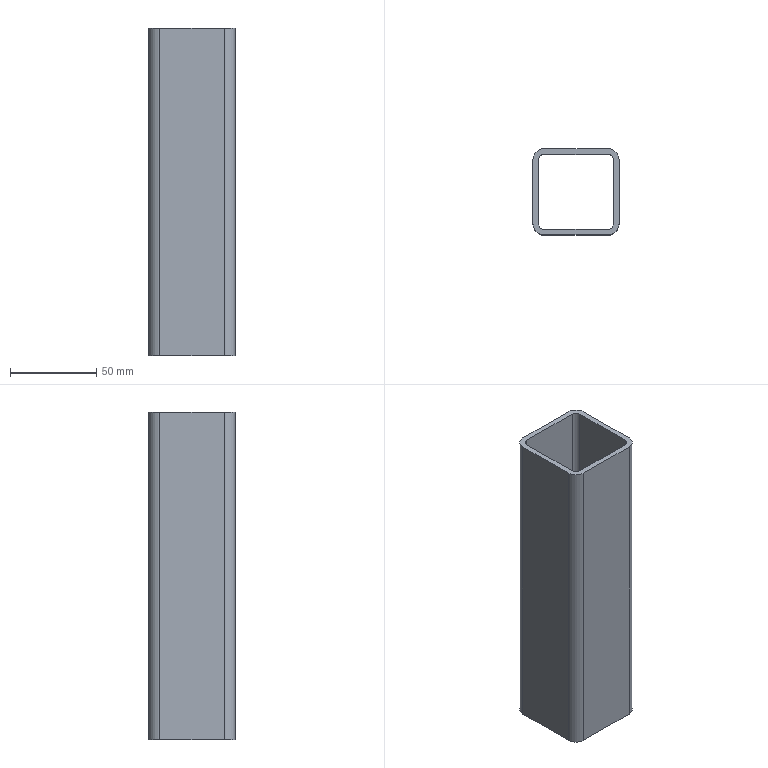Part | STEP file | JIS G 3466 50 x 50 x 3,2 1784904759157 | 1 solid | 18 faces | box 50 x 50 x 190 mm | volume 108807 mm3 | plane 10 | cylinder 8 | commonest cylinder face diameters 6.4 x4 12.8 x4
STEP:
#1=CARTESIAN_POINT('',(-18.6,-21.8,240.));
#2=VERTEX_POINT('',#1);
#3=CARTESIAN_POINT('',(18.6,-21.8,240.));
#4=VERTEX_POINT('',#3);
#5=CARTESIAN_POINT('',(9.3,-21.8,240.));
#6=DIRECTION('',(1.,0.,0.));
#7=VECTOR('',#6,10.);
#8=LINE('',#5,#7);
#9=EDGE_CURVE('',#2,#4,#8,.T.);
#10=ORIENTED_EDGE('',*,*,#9,.T.);
#11=CARTESIAN_POINT('',(18.6,-21.8,50.));
#12=VERTEX_POINT('',#11);
#13=CARTESIAN_POINT('',(18.6,-21.8,0.));
#14=DIRECTION('',(0.,0.,1.));
#15=VECTOR('',#14,10.);
#16=LINE('',#13,#15);
#17=EDGE_CURVE('',#12,#4,#16,.T.);
#18=ORIENTED_EDGE('',*,*,#17,.F.);
#19=CARTESIAN_POINT('',(-18.6,-21.8,50.));
#20=VERTEX_POINT('',#19);
#21=CARTESIAN_POINT('',(9.3,-21.8,50.));
#22=DIRECTION('',(1.,0.,0.));
#23=VECTOR('',#22,10.);
#24=LINE('',#21,#23);
#25=EDGE_CURVE('',#20,#12,#24,.T.);
#26=ORIENTED_EDGE('',*,*,#25,.F.);
#27=CARTESIAN_POINT('',(-18.6,-21.8,0.));
#28=DIRECTION('',(0.,0.,1.));
#29=VECTOR('',#28,10.);
#30=LINE('',#27,#29);
#31=EDGE_CURVE('',#20,#2,#30,.T.);
#32=ORIENTED_EDGE('',*,*,#31,.T.);
#33=EDGE_LOOP('',(#10,#18,#26,#32));
#34=FACE_OUTER_BOUND('',#33,.T.);
#35=CARTESIAN_POINT('',(18.6,-21.8,0.));
#36=DIRECTION('',(0.,-1.,0.));
#37=DIRECTION('',(0.,0.,-1.));
#38=AXIS2_PLACEMENT_3D('',#35,#36,#37);
#39=PLANE('',#38);
#40=ADVANCED_FACE('',(#34),#39,.F.);
#41=CARTESIAN_POINT('',(21.8,-18.6,240.));
#42=VERTEX_POINT('',#41);
#43=CARTESIAN_POINT('',(18.6,-18.6,240.));
#44=DIRECTION('',(0.,0.,1.));
#45=DIRECTION('',(0.,1.,0.));
#46=AXIS2_PLACEMENT_3D('',#43,#44,#45);
#47=CIRCLE('',#46,3.2);
#48=EDGE_CURVE('',#4,#42,#47,.T.);
#49=ORIENTED_EDGE('',*,*,#48,.T.);
#50=CARTESIAN_POINT('',(21.8,-18.6,50.));
#51=VERTEX_POINT('',#50);
#52=CARTESIAN_POINT('',(21.8,-18.6,0.));
#53=DIRECTION('',(0.,0.,1.));
#54=VECTOR('',#53,10.);
#55=LINE('',#52,#54);
#56=EDGE_CURVE('',#51,#42,#55,.T.);
#57=ORIENTED_EDGE('',*,*,#56,.F.);
#58=CARTESIAN_POINT('',(18.6,-18.6,50.));
#59=DIRECTION('',(0.,0.,1.));
#60=DIRECTION('',(0.,1.,0.));
#61=AXIS2_PLACEMENT_3D('',#58,#59,#60);
#62=CIRCLE('',#61,3.2);
#63=EDGE_CURVE('',#12,#51,#62,.T.);
#64=ORIENTED_EDGE('',*,*,#63,.F.);
#65=ORIENTED_EDGE('',*,*,#17,.T.);
#66=EDGE_LOOP('',(#49,#57,#64,#65));
#67=FACE_OUTER_BOUND('',#66,.T.);
#68=CARTESIAN_POINT('',(18.6,-18.6,0.));
#69=DIRECTION('',(0.,0.,1.));
#70=DIRECTION('',(0.,1.,0.));
#71=AXIS2_PLACEMENT_3D('',#68,#69,#70);
#72=CYLINDRICAL_SURFACE('',#71,3.2);
#73=ADVANCED_FACE('',(#67),#72,.F.);
#74=CARTESIAN_POINT('',(21.8,18.6,240.));
#75=VERTEX_POINT('',#74);
#76=CARTESIAN_POINT('',(21.8,9.3,240.));
#77=DIRECTION('',(0.,1.,0.));
#78=VECTOR('',#77,10.);
#79=LINE('',#76,#78);
#80=EDGE_CURVE('',#42,#75,#79,.T.);
#81=ORIENTED_EDGE('',*,*,#80,.T.);
#82=CARTESIAN_POINT('',(21.8,18.6,50.));
#83=VERTEX_POINT('',#82);
#84=CARTESIAN_POINT('',(21.8,18.6,0.));
#85=DIRECTION('',(0.,0.,1.));
#86=VECTOR('',#85,10.);
#87=LINE('',#84,#86);
#88=EDGE_CURVE('',#83,#75,#87,.T.);
#89=ORIENTED_EDGE('',*,*,#88,.F.);
#90=CARTESIAN_POINT('',(21.8,9.3,50.));
#91=DIRECTION('',(0.,1.,0.));
#92=VECTOR('',#91,10.);
#93=LINE('',#90,#92);
#94=EDGE_CURVE('',#51,#83,#93,.T.);
#95=ORIENTED_EDGE('',*,*,#94,.F.);
#96=ORIENTED_EDGE('',*,*,#56,.T.);
#97=EDGE_LOOP('',(#81,#89,#95,#96));
#98=FACE_OUTER_BOUND('',#97,.T.);
#99=CARTESIAN_POINT('',(21.8,18.6,0.));
#100=DIRECTION('',(1.,0.,0.));
#101=DIRECTION('',(0.,0.,-1.));
#102=AXIS2_PLACEMENT_3D('',#99,#100,#101);
#103=PLANE('',#102);
#104=ADVANCED_FACE('',(#98),#103,.F.);
#105=CARTESIAN_POINT('',(18.6,21.8,240.));
#106=VERTEX_POINT('',#105);
#107=CARTESIAN_POINT('',(18.6,18.6,240.));
#108=DIRECTION('',(0.,0.,1.));
#109=DIRECTION('',(-1.,0.,0.));
#110=AXIS2_PLACEMENT_3D('',#107,#108,#109);
#111=CIRCLE('',#110,3.2);
#112=EDGE_CURVE('',#75,#106,#111,.T.);
#113=ORIENTED_EDGE('',*,*,#112,.T.);
#114=CARTESIAN_POINT('',(18.6,21.8,50.));
#115=VERTEX_POINT('',#114);
#116=CARTESIAN_POINT('',(18.6,21.8,0.));
#117=DIRECTION('',(0.,0.,1.));
#118=VECTOR('',#117,10.);
#119=LINE('',#116,#118);
#120=EDGE_CURVE('',#115,#106,#119,.T.);
#121=ORIENTED_EDGE('',*,*,#120,.F.);
#122=CARTESIAN_POINT('',(18.6,18.6,50.));
#123=DIRECTION('',(0.,0.,1.));
#124=DIRECTION('',(-1.,0.,0.));
#125=AXIS2_PLACEMENT_3D('',#122,#123,#124);
#126=CIRCLE('',#125,3.2);
#127=EDGE_CURVE('',#83,#115,#126,.T.);
#128=ORIENTED_EDGE('',*,*,#127,.F.);
#129=ORIENTED_EDGE('',*,*,#88,.T.);
#130=EDGE_LOOP('',(#113,#121,#128,#129));
#131=FACE_OUTER_BOUND('',#130,.T.);
#132=CARTESIAN_POINT('',(18.6,18.6,0.));
#133=DIRECTION('',(0.,0.,1.));
#134=DIRECTION('',(-1.,0.,0.));
#135=AXIS2_PLACEMENT_3D('',#132,#133,#134);
#136=CYLINDRICAL_SURFACE('',#135,3.2);
#137=ADVANCED_FACE('',(#131),#136,.F.);
#138=CARTESIAN_POINT('',(25.,18.6,240.));
#139=VERTEX_POINT('',#138);
#140=CARTESIAN_POINT('',(25.,-18.6,240.));
#141=VERTEX_POINT('',#140);
#142=CARTESIAN_POINT('',(25.,9.3,240.));
#143=DIRECTION('',(0.,-1.,0.));
#144=VECTOR('',#143,10.);
#145=LINE('',#142,#144);
#146=EDGE_CURVE('',#139,#141,#145,.T.);
#147=ORIENTED_EDGE('',*,*,#146,.T.);
#148=CARTESIAN_POINT('',(25.,-18.6,50.));
#149=VERTEX_POINT('',#148);
#150=CARTESIAN_POINT('',(25.,-18.6,0.));
#151=DIRECTION('',(0.,0.,1.));
#152=VECTOR('',#151,10.);
#153=LINE('',#150,#152);
#154=EDGE_CURVE('',#149,#141,#153,.T.);
#155=ORIENTED_EDGE('',*,*,#154,.F.);
#156=CARTESIAN_POINT('',(25.,18.6,50.));
#157=VERTEX_POINT('',#156);
#158=CARTESIAN_POINT('',(25.,9.3,50.));
#159=DIRECTION('',(0.,-1.,0.));
#160=VECTOR('',#159,10.);
#161=LINE('',#158,#160);
#162=EDGE_CURVE('',#157,#149,#161,.T.);
#163=ORIENTED_EDGE('',*,*,#162,.F.);
#164=CARTESIAN_POINT('',(25.,18.6,0.));
#165=DIRECTION('',(0.,0.,1.));
#166=VECTOR('',#165,10.);
#167=LINE('',#164,#166);
#168=EDGE_CURVE('',#157,#139,#167,.T.);
#169=ORIENTED_EDGE('',*,*,#168,.T.);
#170=EDGE_LOOP('',(#147,#155,#163,#169));
#171=FACE_OUTER_BOUND('',#170,.T.);
#172=CARTESIAN_POINT('',(25.,18.6,0.));
#173=DIRECTION('',(1.,0.,0.));
#174=DIRECTION('',(0.,0.,-1.));
#175=AXIS2_PLACEMENT_3D('',#172,#173,#174);
#176=PLANE('',#175);
#177=ADVANCED_FACE('',(#171),#176,.T.);
#178=CARTESIAN_POINT('',(18.6,-25.,240.));
#179=VERTEX_POINT('',#178);
#180=CARTESIAN_POINT('',(18.6,-18.6,240.));
#181=DIRECTION('',(0.,0.,-1.));
#182=DIRECTION('',(0.,1.,0.));
#183=AXIS2_PLACEMENT_3D('',#180,#181,#182);
#184=CIRCLE('',#183,6.4);
#185=EDGE_CURVE('',#141,#179,#184,.T.);
#186=ORIENTED_EDGE('',*,*,#185,.T.);
#187=CARTESIAN_POINT('',(18.6,-25.,50.));
#188=VERTEX_POINT('',#187);
#189=CARTESIAN_POINT('',(18.6,-25.,0.));
#190=DIRECTION('',(0.,0.,1.));
#191=VECTOR('',#190,10.);
#192=LINE('',#189,#191);
#193=EDGE_CURVE('',#188,#179,#192,.T.);
#194=ORIENTED_EDGE('',*,*,#193,.F.);
#195=CARTESIAN_POINT('',(18.6,-18.6,50.));
#196=DIRECTION('',(0.,0.,-1.));
#197=DIRECTION('',(0.,1.,0.));
#198=AXIS2_PLACEMENT_3D('',#195,#196,#197);
#199=CIRCLE('',#198,6.4);
#200=EDGE_CURVE('',#149,#188,#199,.T.);
#201=ORIENTED_EDGE('',*,*,#200,.F.);
#202=ORIENTED_EDGE('',*,*,#154,.T.);
#203=EDGE_LOOP('',(#186,#194,#201,#202));
#204=FACE_OUTER_BOUND('',#203,.T.);
#205=CARTESIAN_POINT('',(18.6,-18.6,0.));
#206=DIRECTION('',(0.,0.,1.));
#207=DIRECTION('',(0.,1.,0.));
#208=AXIS2_PLACEMENT_3D('',#205,#206,#207);
#209=CYLINDRICAL_SURFACE('',#208,6.4);
#210=ADVANCED_FACE('',(#204),#209,.T.);
#211=CARTESIAN_POINT('',(-18.6,-25.,240.));
#212=VERTEX_POINT('',#211);
#213=CARTESIAN_POINT('',(9.3,-25.,240.));
#214=DIRECTION('',(-1.,0.,0.));
#215=VECTOR('',#214,10.);
#216=LINE('',#213,#215);
#217=EDGE_CURVE('',#179,#212,#216,.T.);
#218=ORIENTED_EDGE('',*,*,#217,.T.);
#219=CARTESIAN_POINT('',(-18.6,-25.,50.));
#220=VERTEX_POINT('',#219);
#221=CARTESIAN_POINT('',(-18.6,-25.,0.));
#222=DIRECTION('',(0.,0.,1.));
#223=VECTOR('',#222,10.);
#224=LINE('',#221,#223);
#225=EDGE_CURVE('',#220,#212,#224,.T.);
#226=ORIENTED_EDGE('',*,*,#225,.F.);
#227=CARTESIAN_POINT('',(9.3,-25.,50.));
#228=DIRECTION('',(-1.,0.,0.));
#229=VECTOR('',#228,10.);
#230=LINE('',#227,#229);
#231=EDGE_CURVE('',#188,#220,#230,.T.);
#232=ORIENTED_EDGE('',*,*,#231,.F.);
#233=ORIENTED_EDGE('',*,*,#193,.T.);
#234=EDGE_LOOP('',(#218,#226,#232,#233));
#235=FACE_OUTER_BOUND('',#234,.T.);
#236=CARTESIAN_POINT('',(18.6,-25.,0.));
#237=DIRECTION('',(0.,-1.,0.));
#238=DIRECTION('',(0.,0.,-1.));
#239=AXIS2_PLACEMENT_3D('',#236,#237,#238);
#240=PLANE('',#239);
#241=ADVANCED_FACE('',(#235),#240,.T.);
#242=CARTESIAN_POINT('',(-25.,-18.6,240.));
#243=VERTEX_POINT('',#242);
#244=CARTESIAN_POINT('',(-18.6,-18.6,240.));
#245=DIRECTION('',(0.,0.,-1.));
#246=DIRECTION('',(1.,0.,0.));
#247=AXIS2_PLACEMENT_3D('',#244,#245,#246);
#248=CIRCLE('',#247,6.4);
#249=EDGE_CURVE('',#212,#243,#248,.T.);
#250=ORIENTED_EDGE('',*,*,#249,.T.);
#251=CARTESIAN_POINT('',(-25.,-18.6,50.));
#252=VERTEX_POINT('',#251);
#253=CARTESIAN_POINT('',(-25.,-18.6,0.));
#254=DIRECTION('',(0.,0.,1.));
#255=VECTOR('',#254,10.);
#256=LINE('',#253,#255);
#257=EDGE_CURVE('',#252,#243,#256,.T.);
#258=ORIENTED_EDGE('',*,*,#257,.F.);
#259=CARTESIAN_POINT('',(-18.6,-18.6,50.));
#260=DIRECTION('',(0.,0.,-1.));
#261=DIRECTION('',(1.,0.,0.));
#262=AXIS2_PLACEMENT_3D('',#259,#260,#261);
#263=CIRCLE('',#262,6.4);
#264=EDGE_CURVE('',#220,#252,#263,.T.);
#265=ORIENTED_EDGE('',*,*,#264,.F.);
#266=ORIENTED_EDGE('',*,*,#225,.T.);
#267=EDGE_LOOP('',(#250,#258,#265,#266));
#268=FACE_OUTER_BOUND('',#267,.T.);
#269=CARTESIAN_POINT('',(-18.6,-18.6,0.));
#270=DIRECTION('',(0.,0.,1.));
#271=DIRECTION('',(1.,0.,0.));
#272=AXIS2_PLACEMENT_3D('',#269,#270,#271);
#273=CYLINDRICAL_SURFACE('',#272,6.4);
#274=ADVANCED_FACE('',(#268),#273,.T.);
#275=CARTESIAN_POINT('',(-18.6,21.8,240.));
#276=VERTEX_POINT('',#275);
#277=CARTESIAN_POINT('',(-9.3,21.8,240.));
#278=DIRECTION('',(-1.,0.,0.));
#279=VECTOR('',#278,10.);
#280=LINE('',#277,#279);
#281=EDGE_CURVE('',#106,#276,#280,.T.);
#282=ORIENTED_EDGE('',*,*,#281,.T.);
#283=CARTESIAN_POINT('',(-18.6,21.8,50.));
#284=VERTEX_POINT('',#283);
#285=CARTESIAN_POINT('',(-18.6,21.8,0.));
#286=DIRECTION('',(0.,0.,1.));
#287=VECTOR('',#286,10.);
#288=LINE('',#285,#287);
#289=EDGE_CURVE('',#284,#276,#288,.T.);
#290=ORIENTED_EDGE('',*,*,#289,.F.);
#291=CARTESIAN_POINT('',(-9.3,21.8,50.));
#292=DIRECTION('',(-1.,0.,0.));
#293=VECTOR('',#292,10.);
#294=LINE('',#291,#293);
#295=EDGE_CURVE('',#115,#284,#294,.T.);
#296=ORIENTED_EDGE('',*,*,#295,.F.);
#297=ORIENTED_EDGE('',*,*,#120,.T.);
#298=EDGE_LOOP('',(#282,#290,#296,#297));
#299=FACE_OUTER_BOUND('',#298,.T.);
#300=CARTESIAN_POINT('',(-18.6,21.8,0.));
#301=DIRECTION('',(0.,1.,0.));
#302=DIRECTION('',(0.,0.,1.));
#303=AXIS2_PLACEMENT_3D('',#300,#301,#302);
#304=PLANE('',#303);
#305=ADVANCED_FACE('',(#299),#304,.F.);
#306=CARTESIAN_POINT('',(-21.8,-18.6,240.));
#307=VERTEX_POINT('',#306);
#308=CARTESIAN_POINT('',(-18.6,-18.6,240.));
#309=DIRECTION('',(0.,0.,1.));
#310=DIRECTION('',(1.,0.,0.));
#311=AXIS2_PLACEMENT_3D('',#308,#309,#310);
#312=CIRCLE('',#311,3.2);
#313=EDGE_CURVE('',#307,#2,#312,.T.);
#314=ORIENTED_EDGE('',*,*,#313,.T.);
#315=ORIENTED_EDGE('',*,*,#31,.F.);
#316=CARTESIAN_POINT('',(-21.8,-18.6,50.));
#317=VERTEX_POINT('',#316);
#318=CARTESIAN_POINT('',(-18.6,-18.6,50.));
#319=DIRECTION('',(0.,0.,1.));
#320=DIRECTION('',(1.,0.,0.));
#321=AXIS2_PLACEMENT_3D('',#318,#319,#320);
#322=CIRCLE('',#321,3.2);
#323=EDGE_CURVE('',#317,#20,#322,.T.);
#324=ORIENTED_EDGE('',*,*,#323,.F.);
#325=CARTESIAN_POINT('',(-21.8,-18.6,0.));
#326=DIRECTION('',(0.,0.,1.));
#327=VECTOR('',#326,10.);
#328=LINE('',#325,#327);
#329=EDGE_CURVE('',#317,#307,#328,.T.);
#330=ORIENTED_EDGE('',*,*,#329,.T.);
#331=EDGE_LOOP('',(#314,#315,#324,#330));
#332=FACE_OUTER_BOUND('',#331,.T.);
#333=CARTESIAN_POINT('',(-18.6,-18.6,0.));
#334=DIRECTION('',(0.,0.,1.));
#335=DIRECTION('',(1.,0.,0.));
#336=AXIS2_PLACEMENT_3D('',#333,#334,#335);
#337=CYLINDRICAL_SURFACE('',#336,3.2);
#338=ADVANCED_FACE('',(#332),#337,.F.);
#339=CARTESIAN_POINT('',(-21.8,18.6,240.));
#340=VERTEX_POINT('',#339);
#341=CARTESIAN_POINT('',(-21.8,-9.3,240.));
#342=DIRECTION('',(0.,-1.,0.));
#343=VECTOR('',#342,10.);
#344=LINE('',#341,#343);
#345=EDGE_CURVE('',#340,#307,#344,.T.);
#346=ORIENTED_EDGE('',*,*,#345,.T.);
#347=ORIENTED_EDGE('',*,*,#329,.F.);
#348=CARTESIAN_POINT('',(-21.8,18.6,50.));
#349=VERTEX_POINT('',#348);
#350=CARTESIAN_POINT('',(-21.8,-9.3,50.));
#351=DIRECTION('',(0.,-1.,0.));
#352=VECTOR('',#351,10.);
#353=LINE('',#350,#352);
#354=EDGE_CURVE('',#349,#317,#353,.T.);
#355=ORIENTED_EDGE('',*,*,#354,.F.);
#356=CARTESIAN_POINT('',(-21.8,18.6,0.));
#357=DIRECTION('',(0.,0.,1.));
#358=VECTOR('',#357,10.);
#359=LINE('',#356,#358);
#360=EDGE_CURVE('',#349,#340,#359,.T.);
#361=ORIENTED_EDGE('',*,*,#360,.T.);
#362=EDGE_LOOP('',(#346,#347,#355,#361));
#363=FACE_OUTER_BOUND('',#362,.T.);
#364=CARTESIAN_POINT('',(-21.8,-18.6,0.));
#365=DIRECTION('',(-1.,0.,0.));
#366=DIRECTION('',(0.,0.,1.));
#367=AXIS2_PLACEMENT_3D('',#364,#365,#366);
#368=PLANE('',#367);
#369=ADVANCED_FACE('',(#363),#368,.F.);
#370=CARTESIAN_POINT('',(-18.6,18.6,240.));
#371=DIRECTION('',(0.,0.,1.));
#372=DIRECTION('',(0.,-1.,0.));
#373=AXIS2_PLACEMENT_3D('',#370,#371,#372);
#374=CIRCLE('',#373,3.2);
#375=EDGE_CURVE('',#276,#340,#374,.T.);
#376=ORIENTED_EDGE('',*,*,#375,.T.);
#377=ORIENTED_EDGE('',*,*,#360,.F.);
#378=CARTESIAN_POINT('',(-18.6,18.6,50.));
#379=DIRECTION('',(0.,0.,1.));
#380=DIRECTION('',(0.,-1.,0.));
#381=AXIS2_PLACEMENT_3D('',#378,#379,#380);
#382=CIRCLE('',#381,3.2);
#383=EDGE_CURVE('',#284,#349,#382,.T.);
#384=ORIENTED_EDGE('',*,*,#383,.F.);
#385=ORIENTED_EDGE('',*,*,#289,.T.);
#386=EDGE_LOOP('',(#376,#377,#384,#385));
#387=FACE_OUTER_BOUND('',#386,.T.);
#388=CARTESIAN_POINT('',(-18.6,18.6,0.));
#389=DIRECTION('',(0.,0.,1.));
#390=DIRECTION('',(0.,-1.,0.));
#391=AXIS2_PLACEMENT_3D('',#388,#389,#390);
#392=CYLINDRICAL_SURFACE('',#391,3.2);
#393=ADVANCED_FACE('',(#387),#392,.F.);
#394=CARTESIAN_POINT('',(-25.,18.6,240.));
#395=VERTEX_POINT('',#394);
#396=CARTESIAN_POINT('',(-25.,-9.3,240.));
#397=DIRECTION('',(0.,1.,0.));
#398=VECTOR('',#397,10.);
#399=LINE('',#396,#398);
#400=EDGE_CURVE('',#243,#395,#399,.T.);
#401=ORIENTED_EDGE('',*,*,#400,.T.);
#402=CARTESIAN_POINT('',(-25.,18.6,50.));
#403=VERTEX_POINT('',#402);
#404=CARTESIAN_POINT('',(-25.,18.6,0.));
#405=DIRECTION('',(0.,0.,1.));
#406=VECTOR('',#405,10.);
#407=LINE('',#404,#406);
#408=EDGE_CURVE('',#403,#395,#407,.T.);
#409=ORIENTED_EDGE('',*,*,#408,.F.);
#410=CARTESIAN_POINT('',(-25.,-9.3,50.));
#411=DIRECTION('',(0.,1.,0.));
#412=VECTOR('',#411,10.);
#413=LINE('',#410,#412);
#414=EDGE_CURVE('',#252,#403,#413,.T.);
#415=ORIENTED_EDGE('',*,*,#414,.F.);
#416=ORIENTED_EDGE('',*,*,#257,.T.);
#417=EDGE_LOOP('',(#401,#409,#415,#416));
#418=FACE_OUTER_BOUND('',#417,.T.);
#419=CARTESIAN_POINT('',(-25.,-18.6,0.));
#420=DIRECTION('',(-1.,0.,0.));
#421=DIRECTION('',(0.,0.,1.));
#422=AXIS2_PLACEMENT_3D('',#419,#420,#421);
#423=PLANE('',#422);
#424=ADVANCED_FACE('',(#418),#423,.T.);
#425=CARTESIAN_POINT('',(-18.6,25.,240.));
#426=VERTEX_POINT('',#425);
#427=CARTESIAN_POINT('',(-18.6,18.6,240.));
#428=DIRECTION('',(0.,0.,-1.));
#429=DIRECTION('',(0.,-1.,0.));
#430=AXIS2_PLACEMENT_3D('',#427,#428,#429);
#431=CIRCLE('',#430,6.4);
#432=EDGE_CURVE('',#395,#426,#431,.T.);
#433=ORIENTED_EDGE('',*,*,#432,.T.);
#434=CARTESIAN_POINT('',(-18.6,25.,50.));
#435=VERTEX_POINT('',#434);
#436=CARTESIAN_POINT('',(-18.6,25.,0.));
#437=DIRECTION('',(0.,0.,1.));
#438=VECTOR('',#437,10.);
#439=LINE('',#436,#438);
#440=EDGE_CURVE('',#435,#426,#439,.T.);
#441=ORIENTED_EDGE('',*,*,#440,.F.);
#442=CARTESIAN_POINT('',(-18.6,18.6,50.));
#443=DIRECTION('',(0.,0.,-1.));
#444=DIRECTION('',(0.,-1.,0.));
#445=AXIS2_PLACEMENT_3D('',#442,#443,#444);
#446=CIRCLE('',#445,6.4);
#447=EDGE_CURVE('',#403,#435,#446,.T.);
#448=ORIENTED_EDGE('',*,*,#447,.F.);
#449=ORIENTED_EDGE('',*,*,#408,.T.);
#450=EDGE_LOOP('',(#433,#441,#448,#449));
#451=FACE_OUTER_BOUND('',#450,.T.);
#452=CARTESIAN_POINT('',(-18.6,18.6,0.));
#453=DIRECTION('',(0.,0.,1.));
#454=DIRECTION('',(0.,-1.,0.));
#455=AXIS2_PLACEMENT_3D('',#452,#453,#454);
#456=CYLINDRICAL_SURFACE('',#455,6.4);
#457=ADVANCED_FACE('',(#451),#456,.T.);
#458=CARTESIAN_POINT('',(18.6,25.,240.));
#459=VERTEX_POINT('',#458);
#460=CARTESIAN_POINT('',(-9.3,25.,240.));
#461=DIRECTION('',(1.,0.,0.));
#462=VECTOR('',#461,10.);
#463=LINE('',#460,#462);
#464=EDGE_CURVE('',#426,#459,#463,.T.);
#465=ORIENTED_EDGE('',*,*,#464,.T.);
#466=CARTESIAN_POINT('',(18.6,25.,50.));
#467=VERTEX_POINT('',#466);
#468=CARTESIAN_POINT('',(18.6,25.,0.));
#469=DIRECTION('',(0.,0.,1.));
#470=VECTOR('',#469,10.);
#471=LINE('',#468,#470);
#472=EDGE_CURVE('',#467,#459,#471,.T.);
#473=ORIENTED_EDGE('',*,*,#472,.F.);
#474=CARTESIAN_POINT('',(-9.3,25.,50.));
#475=DIRECTION('',(1.,0.,0.));
#476=VECTOR('',#475,10.);
#477=LINE('',#474,#476);
#478=EDGE_CURVE('',#435,#467,#477,.T.);
#479=ORIENTED_EDGE('',*,*,#478,.F.);
#480=ORIENTED_EDGE('',*,*,#440,.T.);
#481=EDGE_LOOP('',(#465,#473,#479,#480));
#482=FACE_OUTER_BOUND('',#481,.T.);
#483=CARTESIAN_POINT('',(-18.6,25.,0.));
#484=DIRECTION('',(0.,1.,0.));
#485=DIRECTION('',(0.,0.,1.));
#486=AXIS2_PLACEMENT_3D('',#483,#484,#485);
#487=PLANE('',#486);
#488=ADVANCED_FACE('',(#482),#487,.T.);
#489=CARTESIAN_POINT('',(18.6,18.6,240.));
#490=DIRECTION('',(0.,0.,-1.));
#491=DIRECTION('',(-1.,0.,0.));
#492=AXIS2_PLACEMENT_3D('',#489,#490,#491);
#493=CIRCLE('',#492,6.4);
#494=EDGE_CURVE('',#459,#139,#493,.T.);
#495=ORIENTED_EDGE('',*,*,#494,.T.);
#496=ORIENTED_EDGE('',*,*,#168,.F.);
#497=CARTESIAN_POINT('',(18.6,18.6,50.));
#498=DIRECTION('',(0.,0.,-1.));
#499=DIRECTION('',(-1.,0.,0.));
#500=AXIS2_PLACEMENT_3D('',#497,#498,#499);
#501=CIRCLE('',#500,6.4);
#502=EDGE_CURVE('',#467,#157,#501,.T.);
#503=ORIENTED_EDGE('',*,*,#502,.F.);
#504=ORIENTED_EDGE('',*,*,#472,.T.);
#505=EDGE_LOOP('',(#495,#496,#503,#504));
#506=FACE_OUTER_BOUND('',#505,.T.);
#507=CARTESIAN_POINT('',(18.6,18.6,0.));
#508=DIRECTION('',(0.,0.,1.));
#509=DIRECTION('',(-1.,0.,0.));
#510=AXIS2_PLACEMENT_3D('',#507,#508,#509);
#511=CYLINDRICAL_SURFACE('',#510,6.4);
#512=ADVANCED_FACE('',(#506),#511,.T.);
#513=ORIENTED_EDGE('',*,*,#414,.T.);
#514=ORIENTED_EDGE('',*,*,#447,.T.);
#515=ORIENTED_EDGE('',*,*,#478,.T.);
#516=ORIENTED_EDGE('',*,*,#502,.T.);
#517=ORIENTED_EDGE('',*,*,#162,.T.);
#518=ORIENTED_EDGE('',*,*,#200,.T.);
#519=ORIENTED_EDGE('',*,*,#231,.T.);
#520=ORIENTED_EDGE('',*,*,#264,.T.);
#521=EDGE_LOOP('',(#513,#514,#515,#516,#517,#518,#519,#520));
#522=FACE_OUTER_BOUND('',#521,.T.);
#523=ORIENTED_EDGE('',*,*,#295,.T.);
#524=ORIENTED_EDGE('',*,*,#383,.T.);
#525=ORIENTED_EDGE('',*,*,#354,.T.);
#526=ORIENTED_EDGE('',*,*,#323,.T.);
#527=ORIENTED_EDGE('',*,*,#25,.T.);
#528=ORIENTED_EDGE('',*,*,#63,.T.);
#529=ORIENTED_EDGE('',*,*,#94,.T.);
#530=ORIENTED_EDGE('',*,*,#127,.T.);
#531=EDGE_LOOP('',(#523,#524,#525,#526,#527,#528,#529,#530));
#532=FACE_BOUND('',#531,.T.);
#533=CARTESIAN_POINT('',(0.,0.,50.));
#534=DIRECTION('',(0.,0.,1.));
#535=DIRECTION('',(1.,0.,0.));
#536=AXIS2_PLACEMENT_3D('',#533,#534,#535);
#537=PLANE('',#536);
#538=ADVANCED_FACE('',(#522,#532),#537,.F.);
#539=ORIENTED_EDGE('',*,*,#400,.F.);
#540=ORIENTED_EDGE('',*,*,#249,.F.);
#541=ORIENTED_EDGE('',*,*,#217,.F.);
#542=ORIENTED_EDGE('',*,*,#185,.F.);
#543=ORIENTED_EDGE('',*,*,#146,.F.);
#544=ORIENTED_EDGE('',*,*,#494,.F.);
#545=ORIENTED_EDGE('',*,*,#464,.F.);
#546=ORIENTED_EDGE('',*,*,#432,.F.);
#547=EDGE_LOOP('',(#539,#540,#541,#542,#543,#544,#545,#546));
#548=FACE_OUTER_BOUND('',#547,.T.);
#549=ORIENTED_EDGE('',*,*,#281,.F.);
#550=ORIENTED_EDGE('',*,*,#112,.F.);
#551=ORIENTED_EDGE('',*,*,#80,.F.);
#552=ORIENTED_EDGE('',*,*,#48,.F.);
#553=ORIENTED_EDGE('',*,*,#9,.F.);
#554=ORIENTED_EDGE('',*,*,#313,.F.);
#555=ORIENTED_EDGE('',*,*,#345,.F.);
#556=ORIENTED_EDGE('',*,*,#375,.F.);
#557=EDGE_LOOP('',(#549,#550,#551,#552,#553,#554,#555,#556));
#558=FACE_BOUND('',#557,.T.);
#559=CARTESIAN_POINT('',(0.,0.,240.));
#560=DIRECTION('',(0.,0.,1.));
#561=DIRECTION('',(1.,0.,0.));
#562=AXIS2_PLACEMENT_3D('',#559,#560,#561);
#563=PLANE('',#562);
#564=ADVANCED_FACE('',(#548,#558),#563,.T.);
#565=CLOSED_SHELL('',(#40,#73,#104,#137,#177,#210,#241,#274,#305,#338,#369,#393,#424,#457,#488,#512,#538,#564));
#566=MANIFOLD_SOLID_BREP('',#565);
#567=(LENGTH_UNIT()NAMED_UNIT(*)SI_UNIT(.MILLI.,.METRE.));
#568=UNCERTAINTY_MEASURE_WITH_UNIT(LENGTH_MEASURE(0.01),#567,'','');
#569=(NAMED_UNIT(*)PLANE_ANGLE_UNIT()SI_UNIT($,.RADIAN.));
#570=(NAMED_UNIT(*)SI_UNIT($,.STERADIAN.)SOLID_ANGLE_UNIT());
#571=(GEOMETRIC_REPRESENTATION_CONTEXT(3)GLOBAL_UNCERTAINTY_ASSIGNED_CONTEXT((#568))GLOBAL_UNIT_ASSIGNED_CONTEXT((#567,#569,#570))REPRESENTATION_CONTEXT('',''));
#572=ADVANCED_BREP_SHAPE_REPRESENTATION('',(#566),#571);